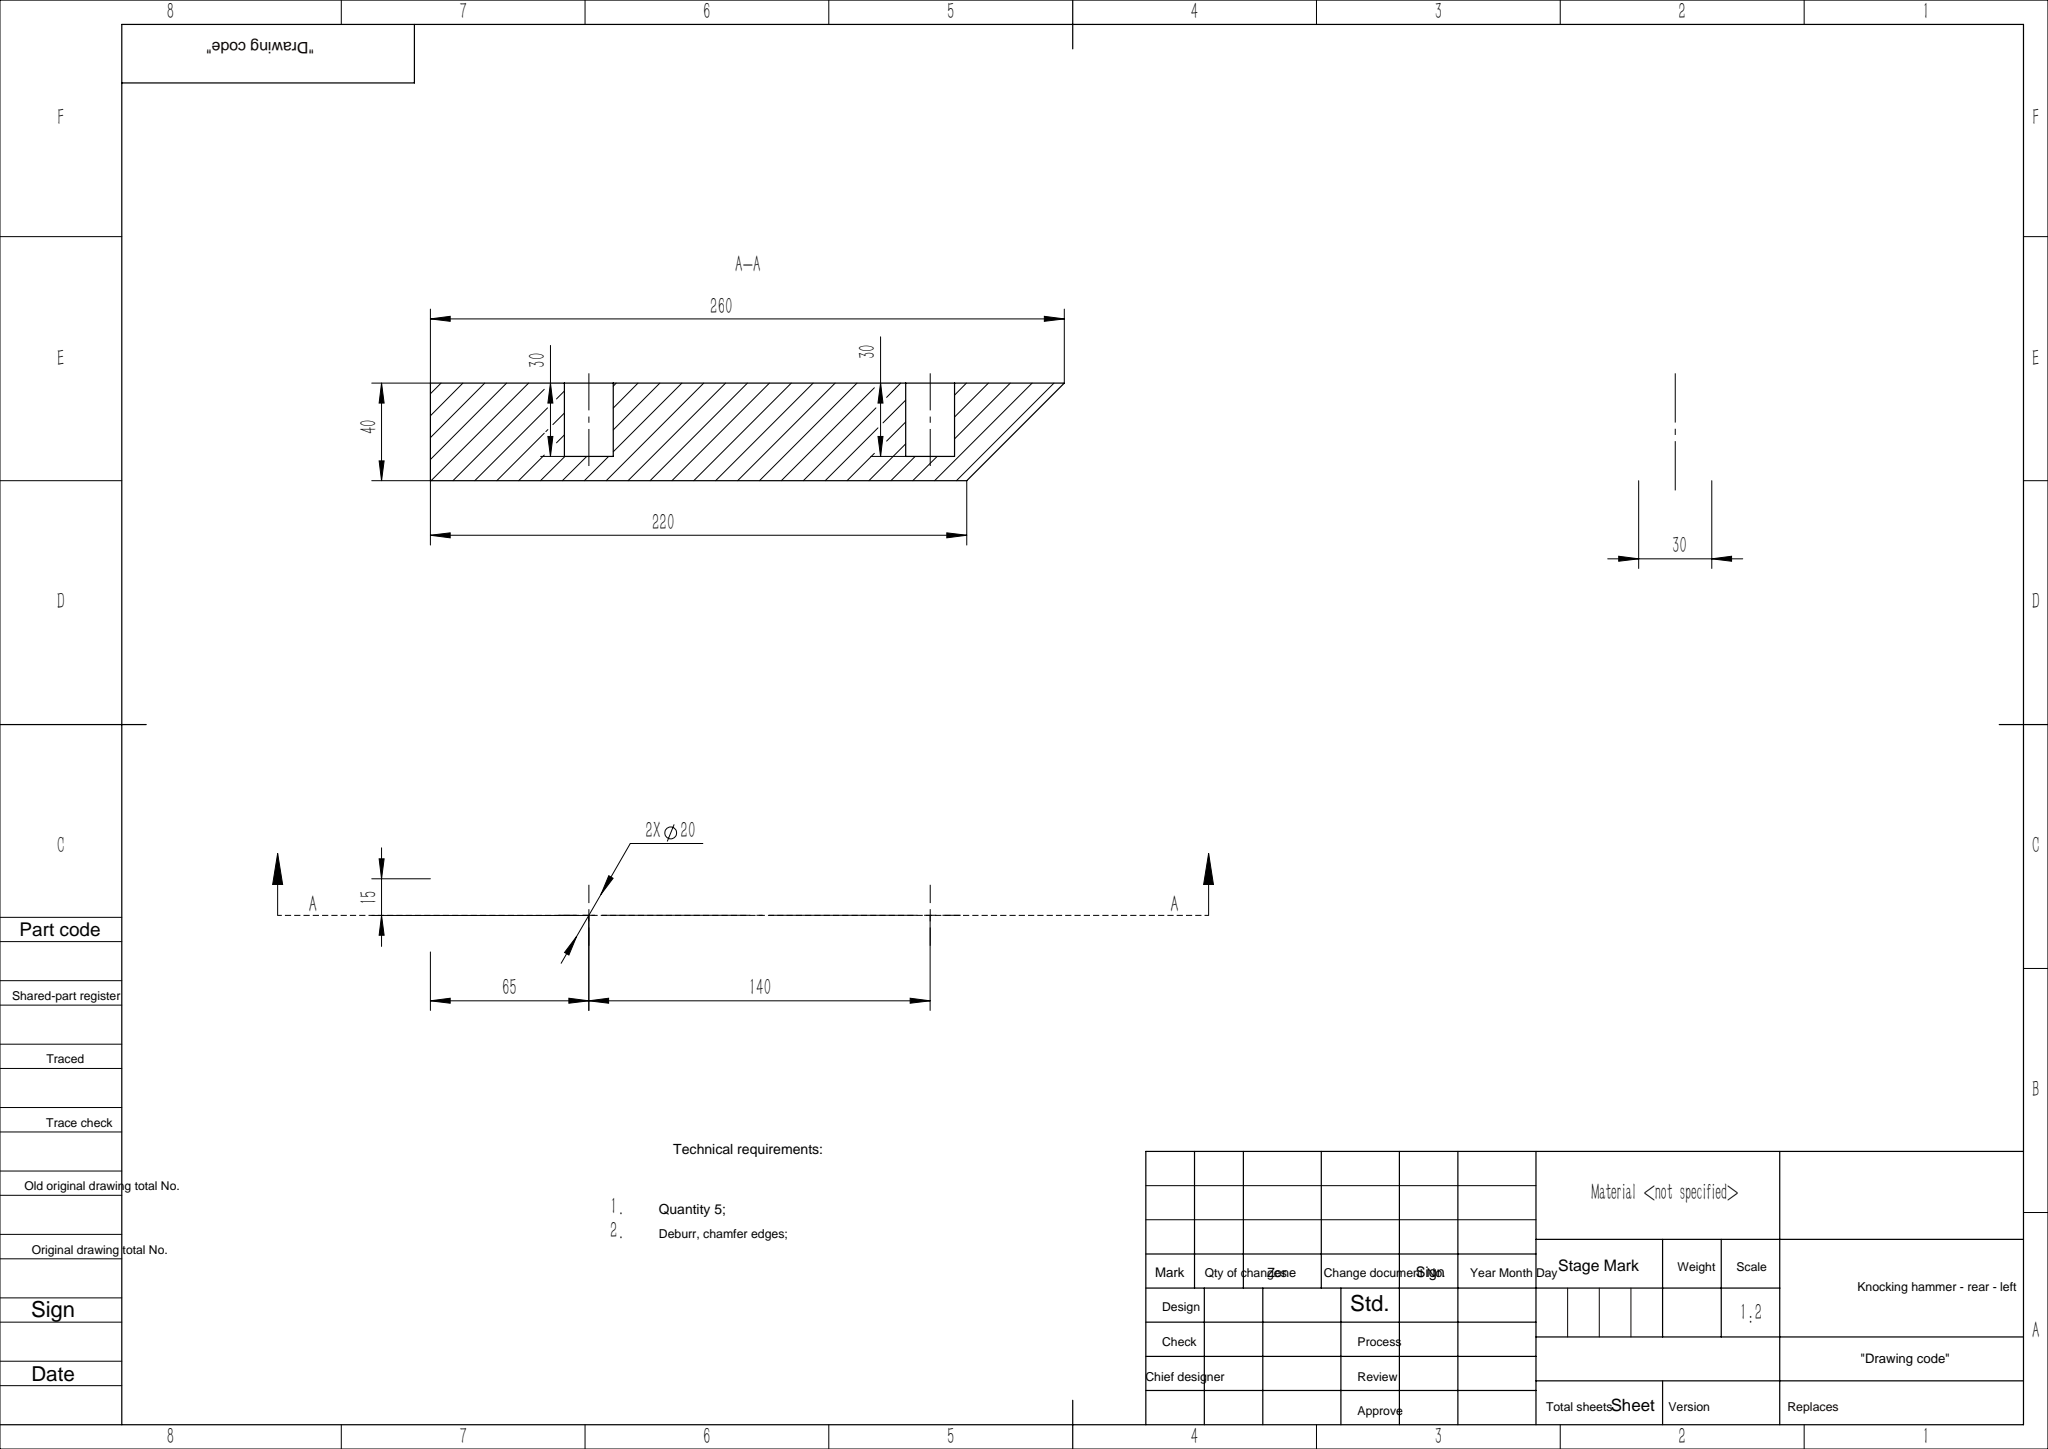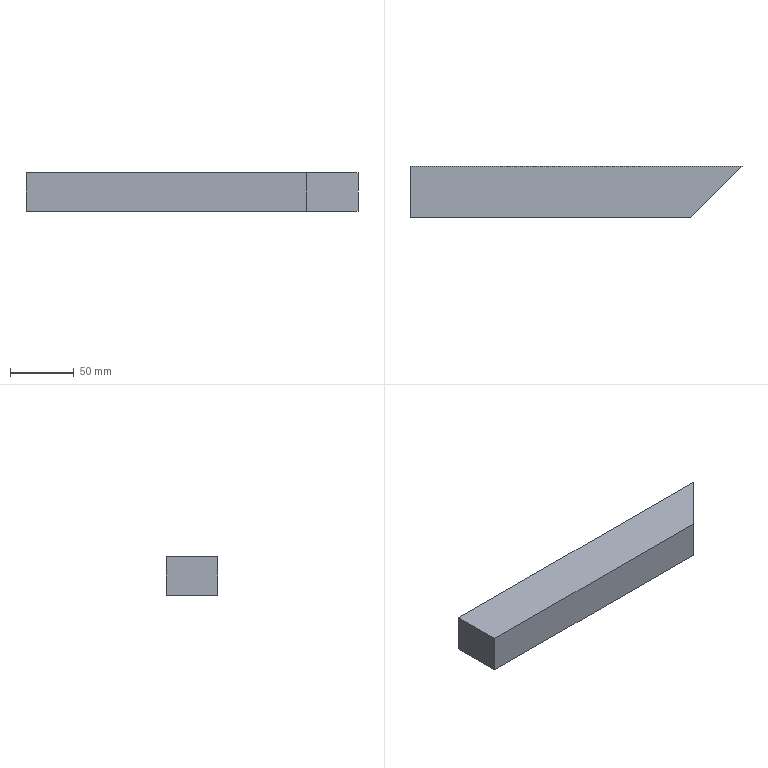Part | SolidWorks | features ICE 3, Extrusion 1 | 1 solid | 12 faces | box 260 x 40 x 30 mm | volume 269150 mm3 | plane 8 | cylinder 4 | commonest cylinder face diameters 20 x4
STEP:
#1=CARTESIAN_POINT('',(-70.,10.,-10.));
#2=VERTEX_POINT('',#1);
#3=CARTESIAN_POINT('',(-70.,10.,10.));
#4=VERTEX_POINT('',#3);
#5=CARTESIAN_POINT('',(-70.,10.,0.));
#6=DIRECTION('',(0.,1.,0.));
#7=DIRECTION('',(0.,0.,-1.));
#8=AXIS2_PLACEMENT_3D('',#5,#6,#7);
#9=CIRCLE('',#8,10.);
#10=EDGE_CURVE('',#2,#4,#9,.T.);
#11=ORIENTED_EDGE('',*,*,#10,.F.);
#12=CARTESIAN_POINT('',(-70.,40.,-10.));
#13=VERTEX_POINT('',#12);
#14=CARTESIAN_POINT('',(-70.,10.,-10.));
#15=DIRECTION('',(0.,1.,0.));
#16=VECTOR('',#15,1000.);
#17=LINE('',#14,#16);
#18=EDGE_CURVE('',#2,#13,#17,.T.);
#19=ORIENTED_EDGE('',*,*,#18,.T.);
#20=CARTESIAN_POINT('',(-70.,40.,10.));
#21=VERTEX_POINT('',#20);
#22=CARTESIAN_POINT('',(-70.,40.,0.));
#23=DIRECTION('',(0.,1.,0.));
#24=DIRECTION('',(0.,0.,-1.));
#25=AXIS2_PLACEMENT_3D('',#22,#23,#24);
#26=CIRCLE('',#25,10.);
#27=EDGE_CURVE('',#13,#21,#26,.T.);
#28=ORIENTED_EDGE('',*,*,#27,.T.);
#29=CARTESIAN_POINT('',(-70.,10.,10.));
#30=DIRECTION('',(0.,1.,0.));
#31=VECTOR('',#30,1000.);
#32=LINE('',#29,#31);
#33=EDGE_CURVE('',#4,#21,#32,.T.);
#34=ORIENTED_EDGE('',*,*,#33,.F.);
#35=EDGE_LOOP('',(#11,#19,#28,#34));
#36=FACE_OUTER_BOUND('',#35,.T.);
#37=CARTESIAN_POINT('',(-70.,10.,0.));
#38=DIRECTION('',(0.,1.,0.));
#39=DIRECTION('',(0.,0.,1.));
#40=AXIS2_PLACEMENT_3D('',#37,#38,#39);
#41=CYLINDRICAL_SURFACE('',#40,10.);
#42=ADVANCED_FACE('',(#36),#41,.F.);
#43=CARTESIAN_POINT('',(70.,10.,-10.));
#44=VERTEX_POINT('',#43);
#45=CARTESIAN_POINT('',(70.,10.,10.));
#46=VERTEX_POINT('',#45);
#47=CARTESIAN_POINT('',(70.,10.,0.));
#48=DIRECTION('',(0.,1.,0.));
#49=DIRECTION('',(0.,0.,1.));
#50=AXIS2_PLACEMENT_3D('',#47,#48,#49);
#51=CIRCLE('',#50,10.);
#52=EDGE_CURVE('',#44,#46,#51,.T.);
#53=ORIENTED_EDGE('',*,*,#52,.F.);
#54=CARTESIAN_POINT('',(70.,40.,-10.));
#55=VERTEX_POINT('',#54);
#56=CARTESIAN_POINT('',(70.,10.,-10.));
#57=DIRECTION('',(0.,1.,0.));
#58=VECTOR('',#57,1000.);
#59=LINE('',#56,#58);
#60=EDGE_CURVE('',#44,#55,#59,.T.);
#61=ORIENTED_EDGE('',*,*,#60,.T.);
#62=CARTESIAN_POINT('',(70.,40.,10.));
#63=VERTEX_POINT('',#62);
#64=CARTESIAN_POINT('',(70.,40.,0.));
#65=DIRECTION('',(0.,1.,0.));
#66=DIRECTION('',(0.,0.,1.));
#67=AXIS2_PLACEMENT_3D('',#64,#65,#66);
#68=CIRCLE('',#67,10.);
#69=EDGE_CURVE('',#55,#63,#68,.T.);
#70=ORIENTED_EDGE('',*,*,#69,.T.);
#71=CARTESIAN_POINT('',(70.,10.,10.));
#72=DIRECTION('',(0.,1.,0.));
#73=VECTOR('',#72,1000.);
#74=LINE('',#71,#73);
#75=EDGE_CURVE('',#46,#63,#74,.T.);
#76=ORIENTED_EDGE('',*,*,#75,.F.);
#77=EDGE_LOOP('',(#53,#61,#70,#76));
#78=FACE_OUTER_BOUND('',#77,.T.);
#79=CARTESIAN_POINT('',(70.,10.,0.));
#80=DIRECTION('',(0.,1.,0.));
#81=DIRECTION('',(0.,0.,1.));
#82=AXIS2_PLACEMENT_3D('',#79,#80,#81);
#83=CYLINDRICAL_SURFACE('',#82,10.);
#84=ADVANCED_FACE('',(#78),#83,.F.);
#85=CARTESIAN_POINT('',(125.,40.,-15.));
#86=VERTEX_POINT('',#85);
#87=CARTESIAN_POINT('',(-135.,40.,-15.));
#88=VERTEX_POINT('',#87);
#89=CARTESIAN_POINT('',(-135.,40.,-15.));
#90=DIRECTION('',(-1.,0.,0.));
#91=VECTOR('',#90,1000.);
#92=LINE('',#89,#91);
#93=EDGE_CURVE('',#86,#88,#92,.T.);
#94=ORIENTED_EDGE('',*,*,#93,.F.);
#95=CARTESIAN_POINT('',(85.,0.,-15.));
#96=VERTEX_POINT('',#95);
#97=CARTESIAN_POINT('',(125.,40.,-15.));
#98=DIRECTION('',(-0.7071,-0.7071,0.));
#99=VECTOR('',#98,1000.);
#100=LINE('',#97,#99);
#101=EDGE_CURVE('',#86,#96,#100,.T.);
#102=ORIENTED_EDGE('',*,*,#101,.T.);
#103=CARTESIAN_POINT('',(-135.,0.,-15.));
#104=VERTEX_POINT('',#103);
#105=CARTESIAN_POINT('',(-135.,0.,-15.));
#106=DIRECTION('',(-1.,0.,0.));
#107=VECTOR('',#106,1000.);
#108=LINE('',#105,#107);
#109=EDGE_CURVE('',#96,#104,#108,.T.);
#110=ORIENTED_EDGE('',*,*,#109,.T.);
#111=CARTESIAN_POINT('',(-135.,40.,-15.));
#112=DIRECTION('',(0.,-1.,0.));
#113=VECTOR('',#112,1000.);
#114=LINE('',#111,#113);
#115=EDGE_CURVE('',#88,#104,#114,.T.);
#116=ORIENTED_EDGE('',*,*,#115,.F.);
#117=EDGE_LOOP('',(#94,#102,#110,#116));
#118=FACE_OUTER_BOUND('',#117,.T.);
#119=CARTESIAN_POINT('',(-135.,40.,-15.));
#120=DIRECTION('',(0.,0.,1.));
#121=DIRECTION('',(1.,0.,0.));
#122=AXIS2_PLACEMENT_3D('',#119,#120,#121);
#123=PLANE('',#122);
#124=ADVANCED_FACE('',(#118),#123,.F.);
#125=CARTESIAN_POINT('',(-135.,0.,15.));
#126=VERTEX_POINT('',#125);
#127=CARTESIAN_POINT('',(85.,0.,15.));
#128=VERTEX_POINT('',#127);
#129=CARTESIAN_POINT('',(-135.,0.,15.));
#130=DIRECTION('',(1.,0.,0.));
#131=VECTOR('',#130,1000.);
#132=LINE('',#129,#131);
#133=EDGE_CURVE('',#126,#128,#132,.T.);
#134=ORIENTED_EDGE('',*,*,#133,.T.);
#135=CARTESIAN_POINT('',(125.,40.,15.));
#136=VERTEX_POINT('',#135);
#137=CARTESIAN_POINT('',(125.,40.,15.));
#138=DIRECTION('',(-0.7071,-0.7071,0.));
#139=VECTOR('',#138,1000.);
#140=LINE('',#137,#139);
#141=EDGE_CURVE('',#136,#128,#140,.T.);
#142=ORIENTED_EDGE('',*,*,#141,.F.);
#143=CARTESIAN_POINT('',(-135.,40.,15.));
#144=VERTEX_POINT('',#143);
#145=CARTESIAN_POINT('',(-135.,40.,15.));
#146=DIRECTION('',(1.,0.,0.));
#147=VECTOR('',#146,1000.);
#148=LINE('',#145,#147);
#149=EDGE_CURVE('',#144,#136,#148,.T.);
#150=ORIENTED_EDGE('',*,*,#149,.F.);
#151=CARTESIAN_POINT('',(-135.,40.,15.));
#152=DIRECTION('',(0.,-1.,0.));
#153=VECTOR('',#152,1000.);
#154=LINE('',#151,#153);
#155=EDGE_CURVE('',#144,#126,#154,.T.);
#156=ORIENTED_EDGE('',*,*,#155,.T.);
#157=EDGE_LOOP('',(#134,#142,#150,#156));
#158=FACE_OUTER_BOUND('',#157,.T.);
#159=CARTESIAN_POINT('',(-135.,40.,15.));
#160=DIRECTION('',(0.,0.,-1.));
#161=DIRECTION('',(-1.,0.,0.));
#162=AXIS2_PLACEMENT_3D('',#159,#160,#161);
#163=PLANE('',#162);
#164=ADVANCED_FACE('',(#158),#163,.F.);
#165=CARTESIAN_POINT('',(70.,40.,0.));
#166=DIRECTION('',(0.,1.,0.));
#167=DIRECTION('',(0.,0.,1.));
#168=AXIS2_PLACEMENT_3D('',#165,#166,#167);
#169=CIRCLE('',#168,10.);
#170=EDGE_CURVE('',#63,#55,#169,.T.);
#171=ORIENTED_EDGE('',*,*,#170,.F.);
#172=ORIENTED_EDGE('',*,*,#69,.F.);
#173=EDGE_LOOP('',(#171,#172));
#174=FACE_BOUND('',#173,.T.);
#175=CARTESIAN_POINT('',(-70.,40.,0.));
#176=DIRECTION('',(0.,1.,0.));
#177=DIRECTION('',(0.,0.,-1.));
#178=AXIS2_PLACEMENT_3D('',#175,#176,#177);
#179=CIRCLE('',#178,10.);
#180=EDGE_CURVE('',#21,#13,#179,.T.);
#181=ORIENTED_EDGE('',*,*,#180,.F.);
#182=ORIENTED_EDGE('',*,*,#27,.F.);
#183=EDGE_LOOP('',(#181,#182));
#184=FACE_BOUND('',#183,.T.);
#185=CARTESIAN_POINT('',(125.,40.,-15.));
#186=DIRECTION('',(0.,0.,1.));
#187=VECTOR('',#186,1000.);
#188=LINE('',#185,#187);
#189=EDGE_CURVE('',#86,#136,#188,.T.);
#190=ORIENTED_EDGE('',*,*,#189,.F.);
#191=ORIENTED_EDGE('',*,*,#93,.T.);
#192=CARTESIAN_POINT('',(-135.,40.,15.));
#193=DIRECTION('',(0.,0.,1.));
#194=VECTOR('',#193,1000.);
#195=LINE('',#192,#194);
#196=EDGE_CURVE('',#88,#144,#195,.T.);
#197=ORIENTED_EDGE('',*,*,#196,.T.);
#198=ORIENTED_EDGE('',*,*,#149,.T.);
#199=EDGE_LOOP('',(#190,#191,#197,#198));
#200=FACE_OUTER_BOUND('',#199,.T.);
#201=CARTESIAN_POINT('',(0.,40.,0.));
#202=DIRECTION('',(0.,-1.,0.));
#203=DIRECTION('',(0.,0.,-1.));
#204=AXIS2_PLACEMENT_3D('',#201,#202,#203);
#205=PLANE('',#204);
#206=ADVANCED_FACE('',(#174,#184,#200),#205,.F.);
#207=CARTESIAN_POINT('',(85.,0.,-15.));
#208=DIRECTION('',(0.,0.,1.));
#209=VECTOR('',#208,1000.);
#210=LINE('',#207,#209);
#211=EDGE_CURVE('',#96,#128,#210,.T.);
#212=ORIENTED_EDGE('',*,*,#211,.T.);
#213=ORIENTED_EDGE('',*,*,#133,.F.);
#214=CARTESIAN_POINT('',(-135.,0.,15.));
#215=DIRECTION('',(0.,0.,1.));
#216=VECTOR('',#215,1000.);
#217=LINE('',#214,#216);
#218=EDGE_CURVE('',#104,#126,#217,.T.);
#219=ORIENTED_EDGE('',*,*,#218,.F.);
#220=ORIENTED_EDGE('',*,*,#109,.F.);
#221=EDGE_LOOP('',(#212,#213,#219,#220));
#222=FACE_OUTER_BOUND('',#221,.T.);
#223=CARTESIAN_POINT('',(0.,0.,0.));
#224=DIRECTION('',(0.,-1.,0.));
#225=DIRECTION('',(0.,0.,-1.));
#226=AXIS2_PLACEMENT_3D('',#223,#224,#225);
#227=PLANE('',#226);
#228=ADVANCED_FACE('',(#222),#227,.T.);
#229=ORIENTED_EDGE('',*,*,#218,.T.);
#230=ORIENTED_EDGE('',*,*,#155,.F.);
#231=ORIENTED_EDGE('',*,*,#196,.F.);
#232=ORIENTED_EDGE('',*,*,#115,.T.);
#233=EDGE_LOOP('',(#229,#230,#231,#232));
#234=FACE_OUTER_BOUND('',#233,.T.);
#235=CARTESIAN_POINT('',(-135.,40.,15.));
#236=DIRECTION('',(1.,0.,0.));
#237=DIRECTION('',(0.,0.,-1.));
#238=AXIS2_PLACEMENT_3D('',#235,#236,#237);
#239=PLANE('',#238);
#240=ADVANCED_FACE('',(#234),#239,.F.);
#241=ORIENTED_EDGE('',*,*,#60,.F.);
#242=CARTESIAN_POINT('',(70.,10.,0.));
#243=DIRECTION('',(0.,1.,0.));
#244=DIRECTION('',(0.,0.,1.));
#245=AXIS2_PLACEMENT_3D('',#242,#243,#244);
#246=CIRCLE('',#245,10.);
#247=EDGE_CURVE('',#46,#44,#246,.T.);
#248=ORIENTED_EDGE('',*,*,#247,.F.);
#249=ORIENTED_EDGE('',*,*,#75,.T.);
#250=ORIENTED_EDGE('',*,*,#170,.T.);
#251=EDGE_LOOP('',(#241,#248,#249,#250));
#252=FACE_OUTER_BOUND('',#251,.T.);
#253=CARTESIAN_POINT('',(70.,10.,0.));
#254=DIRECTION('',(0.,1.,0.));
#255=DIRECTION('',(0.,0.,1.));
#256=AXIS2_PLACEMENT_3D('',#253,#254,#255);
#257=CYLINDRICAL_SURFACE('',#256,10.);
#258=ADVANCED_FACE('',(#252),#257,.F.);
#259=ORIENTED_EDGE('',*,*,#247,.T.);
#260=ORIENTED_EDGE('',*,*,#52,.T.);
#261=EDGE_LOOP('',(#259,#260));
#262=FACE_OUTER_BOUND('',#261,.T.);
#263=CARTESIAN_POINT('',(70.,10.,0.));
#264=DIRECTION('',(0.,1.,0.));
#265=DIRECTION('',(0.,0.,1.));
#266=AXIS2_PLACEMENT_3D('',#263,#264,#265);
#267=PLANE('',#266);
#268=ADVANCED_FACE('',(#262),#267,.T.);
#269=ORIENTED_EDGE('',*,*,#18,.F.);
#270=CARTESIAN_POINT('',(-70.,10.,0.));
#271=DIRECTION('',(0.,1.,0.));
#272=DIRECTION('',(0.,0.,-1.));
#273=AXIS2_PLACEMENT_3D('',#270,#271,#272);
#274=CIRCLE('',#273,10.);
#275=EDGE_CURVE('',#4,#2,#274,.T.);
#276=ORIENTED_EDGE('',*,*,#275,.F.);
#277=ORIENTED_EDGE('',*,*,#33,.T.);
#278=ORIENTED_EDGE('',*,*,#180,.T.);
#279=EDGE_LOOP('',(#269,#276,#277,#278));
#280=FACE_OUTER_BOUND('',#279,.T.);
#281=CARTESIAN_POINT('',(-70.,10.,0.));
#282=DIRECTION('',(0.,1.,0.));
#283=DIRECTION('',(0.,0.,1.));
#284=AXIS2_PLACEMENT_3D('',#281,#282,#283);
#285=CYLINDRICAL_SURFACE('',#284,10.);
#286=ADVANCED_FACE('',(#280),#285,.F.);
#287=ORIENTED_EDGE('',*,*,#275,.T.);
#288=ORIENTED_EDGE('',*,*,#10,.T.);
#289=EDGE_LOOP('',(#287,#288));
#290=FACE_OUTER_BOUND('',#289,.T.);
#291=CARTESIAN_POINT('',(-70.,10.,0.));
#292=DIRECTION('',(0.,-1.,0.));
#293=DIRECTION('',(0.,0.,-1.));
#294=AXIS2_PLACEMENT_3D('',#291,#292,#293);
#295=PLANE('',#294);
#296=ADVANCED_FACE('',(#290),#295,.F.);
#297=ORIENTED_EDGE('',*,*,#141,.T.);
#298=ORIENTED_EDGE('',*,*,#211,.F.);
#299=ORIENTED_EDGE('',*,*,#101,.F.);
#300=ORIENTED_EDGE('',*,*,#189,.T.);
#301=EDGE_LOOP('',(#297,#298,#299,#300));
#302=FACE_OUTER_BOUND('',#301,.T.);
#303=CARTESIAN_POINT('',(125.,40.,-15.));
#304=DIRECTION('',(-0.7071,0.7071,0.));
#305=DIRECTION('',(-0.7071,-0.7071,0.));
#306=AXIS2_PLACEMENT_3D('',#303,#304,#305);
#307=PLANE('',#306);
#308=ADVANCED_FACE('',(#302),#307,.F.);
#309=CLOSED_SHELL('',(#42,#84,#124,#164,#206,#228,#240,#258,#268,#286,#296,#308));
#310=MANIFOLD_SOLID_BREP('',#309);
#311=CARTESIAN_POINT('',(0.,0.,0.));
#312=DIRECTION('',(0.,0.,1.));
#313=DIRECTION('',(1.,0.,0.));
#314=AXIS2_PLACEMENT_3D('',#311,#312,#313);
#315=(LENGTH_UNIT()NAMED_UNIT(*)SI_UNIT(.MILLI.,.METRE.));
#316=UNCERTAINTY_MEASURE_WITH_UNIT(LENGTH_MEASURE(0.00001),#315,'','');
#317=(NAMED_UNIT(*)PLANE_ANGLE_UNIT()SI_UNIT($,.RADIAN.));
#318=(NAMED_UNIT(*)SI_UNIT($,.STERADIAN.)SOLID_ANGLE_UNIT());
#319=(GEOMETRIC_REPRESENTATION_CONTEXT(3)GLOBAL_UNCERTAINTY_ASSIGNED_CONTEXT((#316))GLOBAL_UNIT_ASSIGNED_CONTEXT((#315,#317,#318))REPRESENTATION_CONTEXT('',''));
#320=ADVANCED_BREP_SHAPE_REPRESENTATION('',(#310,#314),#319);